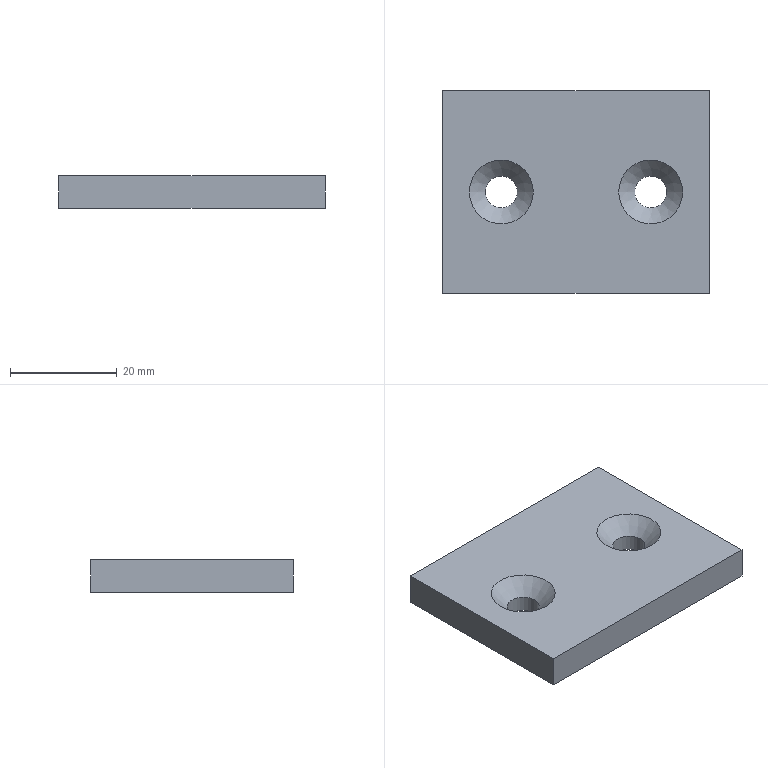Part | NX | features DATUM_CSYS 3, CSUNK_HOLE 2, SKETCH 2, EXTRUDE 1, HOLE PACKAGE 1 | 1 solid | 10 faces | box 50 x 38 x 6 mm | volume 10835 mm3 | plane 6 | cylinder 2 | cone 2 | commonest cylinder face diameters 6 x2
STEP:
#1=CARTESIAN_POINT('',(-25.,-19.,0.));
#2=VERTEX_POINT('',#1);
#3=CARTESIAN_POINT('',(25.,-19.,0.));
#4=VERTEX_POINT('',#3);
#5=CARTESIAN_POINT('',(-25.,-19.,0.));
#6=DIRECTION('',(1.,0.,0.));
#7=VECTOR('',#6,1000.);
#8=LINE('',#5,#7);
#9=EDGE_CURVE('',#2,#4,#8,.T.);
#10=ORIENTED_EDGE('',*,*,#9,.T.);
#11=CARTESIAN_POINT('',(25.,-19.,6.));
#12=VERTEX_POINT('',#11);
#13=CARTESIAN_POINT('',(25.,-19.,6.));
#14=DIRECTION('',(0.,0.,-1.));
#15=VECTOR('',#14,1000.);
#16=LINE('',#13,#15);
#17=EDGE_CURVE('',#12,#4,#16,.T.);
#18=ORIENTED_EDGE('',*,*,#17,.F.);
#19=CARTESIAN_POINT('',(-25.,-19.,6.));
#20=VERTEX_POINT('',#19);
#21=CARTESIAN_POINT('',(-25.,-19.,6.));
#22=DIRECTION('',(1.,0.,0.));
#23=VECTOR('',#22,1000.);
#24=LINE('',#21,#23);
#25=EDGE_CURVE('',#20,#12,#24,.T.);
#26=ORIENTED_EDGE('',*,*,#25,.F.);
#27=CARTESIAN_POINT('',(-25.,-19.,6.));
#28=DIRECTION('',(0.,0.,-1.));
#29=VECTOR('',#28,1000.);
#30=LINE('',#27,#29);
#31=EDGE_CURVE('',#20,#2,#30,.T.);
#32=ORIENTED_EDGE('',*,*,#31,.T.);
#33=EDGE_LOOP('',(#10,#18,#26,#32));
#34=FACE_BOUND('',#33,.T.);
#35=CARTESIAN_POINT('',(-25.,-19.,6.));
#36=DIRECTION('',(0.,1.,0.));
#37=DIRECTION('',(0.,0.,1.));
#38=AXIS2_PLACEMENT_3D('',#35,#36,#37);
#39=PLANE('',#38);
#40=ADVANCED_FACE('',(#34),#39,.F.);
#41=CARTESIAN_POINT('',(25.,19.,0.));
#42=VERTEX_POINT('',#41);
#43=CARTESIAN_POINT('',(25.,-19.,0.));
#44=DIRECTION('',(0.,1.,0.));
#45=VECTOR('',#44,1000.);
#46=LINE('',#43,#45);
#47=EDGE_CURVE('',#4,#42,#46,.T.);
#48=ORIENTED_EDGE('',*,*,#47,.T.);
#49=CARTESIAN_POINT('',(25.,19.,6.));
#50=VERTEX_POINT('',#49);
#51=CARTESIAN_POINT('',(25.,19.,6.));
#52=DIRECTION('',(0.,0.,-1.));
#53=VECTOR('',#52,1000.);
#54=LINE('',#51,#53);
#55=EDGE_CURVE('',#50,#42,#54,.T.);
#56=ORIENTED_EDGE('',*,*,#55,.F.);
#57=CARTESIAN_POINT('',(25.,-19.,6.));
#58=DIRECTION('',(0.,1.,0.));
#59=VECTOR('',#58,1000.);
#60=LINE('',#57,#59);
#61=EDGE_CURVE('',#12,#50,#60,.T.);
#62=ORIENTED_EDGE('',*,*,#61,.F.);
#63=ORIENTED_EDGE('',*,*,#17,.T.);
#64=EDGE_LOOP('',(#48,#56,#62,#63));
#65=FACE_BOUND('',#64,.T.);
#66=CARTESIAN_POINT('',(25.,-19.,6.));
#67=DIRECTION('',(-1.,0.,0.));
#68=DIRECTION('',(0.,0.,1.));
#69=AXIS2_PLACEMENT_3D('',#66,#67,#68);
#70=PLANE('',#69);
#71=ADVANCED_FACE('',(#65),#70,.F.);
#72=CARTESIAN_POINT('',(-25.,19.,0.));
#73=VERTEX_POINT('',#72);
#74=CARTESIAN_POINT('',(25.,19.,0.));
#75=DIRECTION('',(-1.,0.,0.));
#76=VECTOR('',#75,1000.);
#77=LINE('',#74,#76);
#78=EDGE_CURVE('',#42,#73,#77,.T.);
#79=ORIENTED_EDGE('',*,*,#78,.T.);
#80=CARTESIAN_POINT('',(-25.,19.,6.));
#81=VERTEX_POINT('',#80);
#82=CARTESIAN_POINT('',(-25.,19.,6.));
#83=DIRECTION('',(0.,0.,-1.));
#84=VECTOR('',#83,1000.);
#85=LINE('',#82,#84);
#86=EDGE_CURVE('',#81,#73,#85,.T.);
#87=ORIENTED_EDGE('',*,*,#86,.F.);
#88=CARTESIAN_POINT('',(25.,19.,6.));
#89=DIRECTION('',(-1.,0.,0.));
#90=VECTOR('',#89,1000.);
#91=LINE('',#88,#90);
#92=EDGE_CURVE('',#50,#81,#91,.T.);
#93=ORIENTED_EDGE('',*,*,#92,.F.);
#94=ORIENTED_EDGE('',*,*,#55,.T.);
#95=EDGE_LOOP('',(#79,#87,#93,#94));
#96=FACE_BOUND('',#95,.T.);
#97=CARTESIAN_POINT('',(25.,19.,6.));
#98=DIRECTION('',(0.,-1.,0.));
#99=DIRECTION('',(0.,0.,-1.));
#100=AXIS2_PLACEMENT_3D('',#97,#98,#99);
#101=PLANE('',#100);
#102=ADVANCED_FACE('',(#96),#101,.F.);
#103=CARTESIAN_POINT('',(-25.,19.,0.));
#104=DIRECTION('',(0.,-1.,0.));
#105=VECTOR('',#104,1000.);
#106=LINE('',#103,#105);
#107=EDGE_CURVE('',#73,#2,#106,.T.);
#108=ORIENTED_EDGE('',*,*,#107,.T.);
#109=ORIENTED_EDGE('',*,*,#31,.F.);
#110=CARTESIAN_POINT('',(-25.,19.,6.));
#111=DIRECTION('',(0.,-1.,0.));
#112=VECTOR('',#111,1000.);
#113=LINE('',#110,#112);
#114=EDGE_CURVE('',#81,#20,#113,.T.);
#115=ORIENTED_EDGE('',*,*,#114,.F.);
#116=ORIENTED_EDGE('',*,*,#86,.T.);
#117=EDGE_LOOP('',(#108,#109,#115,#116));
#118=FACE_BOUND('',#117,.T.);
#119=CARTESIAN_POINT('',(-25.,19.,6.));
#120=DIRECTION('',(1.,0.,0.));
#121=DIRECTION('',(0.,0.,-1.));
#122=AXIS2_PLACEMENT_3D('',#119,#120,#121);
#123=PLANE('',#122);
#124=ADVANCED_FACE('',(#118),#123,.F.);
#125=CARTESIAN_POINT('',(8.,0.,6.));
#126=VERTEX_POINT('',#125);
#127=CARTESIAN_POINT('',(14.,0.,6.));
#128=DIRECTION('',(0.,0.,-1.));
#129=DIRECTION('',(-1.,0.,0.));
#130=AXIS2_PLACEMENT_3D('',#127,#128,#129);
#131=CIRCLE('',#130,6.);
#132=EDGE_CURVE('',#126,#126,#131,.T.);
#133=ORIENTED_EDGE('',*,*,#132,.T.);
#134=EDGE_LOOP('',(#133));
#135=FACE_BOUND('',#134,.T.);
#136=CARTESIAN_POINT('',(-20.,0.,6.));
#137=VERTEX_POINT('',#136);
#138=CARTESIAN_POINT('',(-14.,0.,6.));
#139=DIRECTION('',(0.,0.,-1.));
#140=DIRECTION('',(-1.,0.,0.));
#141=AXIS2_PLACEMENT_3D('',#138,#139,#140);
#142=CIRCLE('',#141,6.);
#143=EDGE_CURVE('',#137,#137,#142,.T.);
#144=ORIENTED_EDGE('',*,*,#143,.T.);
#145=EDGE_LOOP('',(#144));
#146=FACE_BOUND('',#145,.T.);
#147=ORIENTED_EDGE('',*,*,#25,.T.);
#148=ORIENTED_EDGE('',*,*,#61,.T.);
#149=ORIENTED_EDGE('',*,*,#92,.T.);
#150=ORIENTED_EDGE('',*,*,#114,.T.);
#151=EDGE_LOOP('',(#147,#148,#149,#150));
#152=FACE_BOUND('',#151,.T.);
#153=CARTESIAN_POINT('',(0.,0.,6.));
#154=DIRECTION('',(0.,0.,1.));
#155=DIRECTION('',(1.,0.,0.));
#156=AXIS2_PLACEMENT_3D('',#153,#154,#155);
#157=PLANE('',#156);
#158=ADVANCED_FACE('',(#135,#146,#152),#157,.T.);
#159=CARTESIAN_POINT('',(17.,0.,0.));
#160=VERTEX_POINT('',#159);
#161=CARTESIAN_POINT('',(14.,0.,0.));
#162=DIRECTION('',(0.,0.,1.));
#163=DIRECTION('',(1.,0.,0.));
#164=AXIS2_PLACEMENT_3D('',#161,#162,#163);
#165=CIRCLE('',#164,3.);
#166=EDGE_CURVE('',#160,#160,#165,.T.);
#167=ORIENTED_EDGE('',*,*,#166,.T.);
#168=EDGE_LOOP('',(#167));
#169=FACE_BOUND('',#168,.T.);
#170=CARTESIAN_POINT('',(-11.,0.,0.));
#171=VERTEX_POINT('',#170);
#172=CARTESIAN_POINT('',(-14.,0.,0.));
#173=DIRECTION('',(0.,0.,1.));
#174=DIRECTION('',(1.,0.,0.));
#175=AXIS2_PLACEMENT_3D('',#172,#173,#174);
#176=CIRCLE('',#175,3.);
#177=EDGE_CURVE('',#171,#171,#176,.T.);
#178=ORIENTED_EDGE('',*,*,#177,.T.);
#179=EDGE_LOOP('',(#178));
#180=FACE_BOUND('',#179,.T.);
#181=ORIENTED_EDGE('',*,*,#9,.F.);
#182=ORIENTED_EDGE('',*,*,#107,.F.);
#183=ORIENTED_EDGE('',*,*,#78,.F.);
#184=ORIENTED_EDGE('',*,*,#47,.F.);
#185=EDGE_LOOP('',(#181,#182,#183,#184));
#186=FACE_BOUND('',#185,.T.);
#187=CARTESIAN_POINT('',(0.,0.,0.));
#188=DIRECTION('',(0.,0.,1.));
#189=DIRECTION('',(1.,0.,0.));
#190=AXIS2_PLACEMENT_3D('',#187,#188,#189);
#191=PLANE('',#190);
#192=ADVANCED_FACE('',(#169,#180,#186),#191,.F.);
#193=CARTESIAN_POINT('',(-17.,0.,3.));
#194=VERTEX_POINT('',#193);
#195=CARTESIAN_POINT('',(-14.,0.,3.));
#196=DIRECTION('',(0.,0.,-1.));
#197=DIRECTION('',(-1.,0.,0.));
#198=AXIS2_PLACEMENT_3D('',#195,#196,#197);
#199=CIRCLE('',#198,3.);
#200=EDGE_CURVE('',#194,#194,#199,.F.);
#201=ORIENTED_EDGE('',*,*,#200,.T.);
#202=EDGE_LOOP('',(#201));
#203=FACE_BOUND('',#202,.T.);
#204=ORIENTED_EDGE('',*,*,#177,.F.);
#205=EDGE_LOOP('',(#204));
#206=FACE_BOUND('',#205,.T.);
#207=CARTESIAN_POINT('',(-14.,0.,-495000.));
#208=DIRECTION('',(0.,0.,-1.));
#209=DIRECTION('',(-1.,0.,0.));
#210=AXIS2_PLACEMENT_3D('',#207,#208,#209);
#211=CYLINDRICAL_SURFACE('',#210,3.);
#212=ADVANCED_FACE('',(#203,#206),#211,.F.);
#213=ORIENTED_EDGE('',*,*,#200,.F.);
#214=EDGE_LOOP('',(#213));
#215=FACE_BOUND('',#214,.T.);
#216=ORIENTED_EDGE('',*,*,#143,.F.);
#217=EDGE_LOOP('',(#216));
#218=FACE_BOUND('',#217,.T.);
#219=CARTESIAN_POINT('',(-14.,0.,6.));
#220=DIRECTION('',(0.,0.,1.));
#221=DIRECTION('',(1.,0.,0.));
#222=AXIS2_PLACEMENT_3D('',#219,#220,#221);
#223=CONICAL_SURFACE('',#222,6.,0.7854);
#224=ADVANCED_FACE('',(#215,#218),#223,.F.);
#225=CARTESIAN_POINT('',(11.,0.,3.));
#226=VERTEX_POINT('',#225);
#227=CARTESIAN_POINT('',(14.,0.,3.));
#228=DIRECTION('',(0.,0.,-1.));
#229=DIRECTION('',(-1.,0.,0.));
#230=AXIS2_PLACEMENT_3D('',#227,#228,#229);
#231=CIRCLE('',#230,3.);
#232=EDGE_CURVE('',#226,#226,#231,.F.);
#233=ORIENTED_EDGE('',*,*,#232,.T.);
#234=EDGE_LOOP('',(#233));
#235=FACE_BOUND('',#234,.T.);
#236=ORIENTED_EDGE('',*,*,#166,.F.);
#237=EDGE_LOOP('',(#236));
#238=FACE_BOUND('',#237,.T.);
#239=CARTESIAN_POINT('',(14.,0.,-495000.));
#240=DIRECTION('',(0.,0.,-1.));
#241=DIRECTION('',(-1.,0.,0.));
#242=AXIS2_PLACEMENT_3D('',#239,#240,#241);
#243=CYLINDRICAL_SURFACE('',#242,3.);
#244=ADVANCED_FACE('',(#235,#238),#243,.F.);
#245=ORIENTED_EDGE('',*,*,#232,.F.);
#246=EDGE_LOOP('',(#245));
#247=FACE_BOUND('',#246,.T.);
#248=ORIENTED_EDGE('',*,*,#132,.F.);
#249=EDGE_LOOP('',(#248));
#250=FACE_BOUND('',#249,.T.);
#251=CARTESIAN_POINT('',(14.,0.,6.));
#252=DIRECTION('',(0.,0.,1.));
#253=DIRECTION('',(1.,0.,0.));
#254=AXIS2_PLACEMENT_3D('',#251,#252,#253);
#255=CONICAL_SURFACE('',#254,6.,0.7854);
#256=ADVANCED_FACE('',(#247,#250),#255,.F.);
#257=CLOSED_SHELL('',(#40,#71,#102,#124,#158,#192,#212,#224,#244,#256));
#258=MANIFOLD_SOLID_BREP('',#257);
#259=(LENGTH_UNIT()NAMED_UNIT(*)SI_UNIT(.MILLI.,.METRE.));
#260=UNCERTAINTY_MEASURE_WITH_UNIT(LENGTH_MEASURE(0.00001),#259,'','');
#261=(NAMED_UNIT(*)PLANE_ANGLE_UNIT()SI_UNIT($,.RADIAN.));
#262=(NAMED_UNIT(*)SI_UNIT($,.STERADIAN.)SOLID_ANGLE_UNIT());
#263=(GEOMETRIC_REPRESENTATION_CONTEXT(3)GLOBAL_UNCERTAINTY_ASSIGNED_CONTEXT((#260))GLOBAL_UNIT_ASSIGNED_CONTEXT((#259,#261,#262))REPRESENTATION_CONTEXT('',''));
#264=ADVANCED_BREP_SHAPE_REPRESENTATION('',(#258),#263);